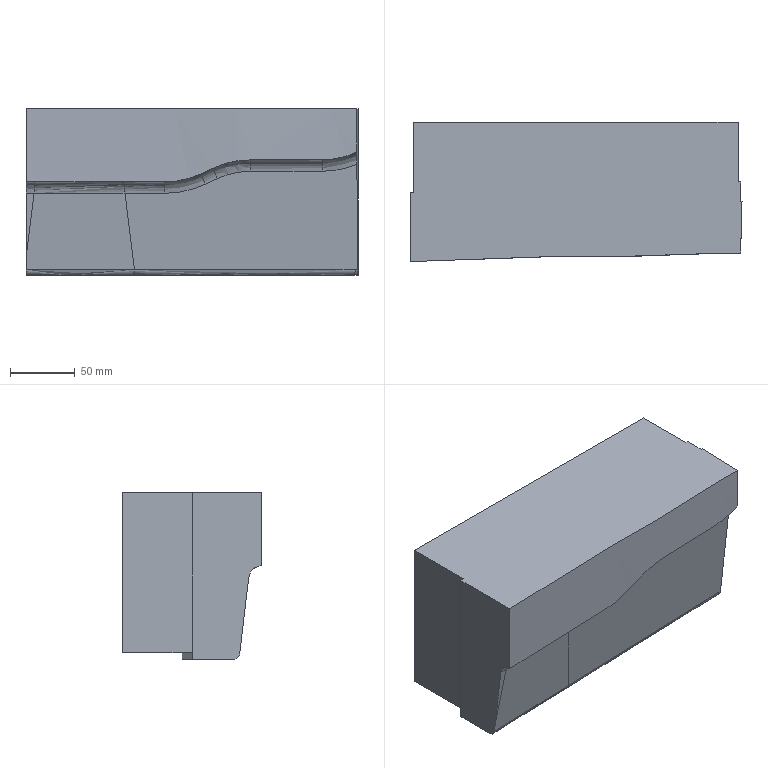Part | NX | features solid 2 | 1 solid | 43 faces | box 256.082 x 107.457 x 128.65 mm | volume 3037942 mm3 | spline 32 | plane 11